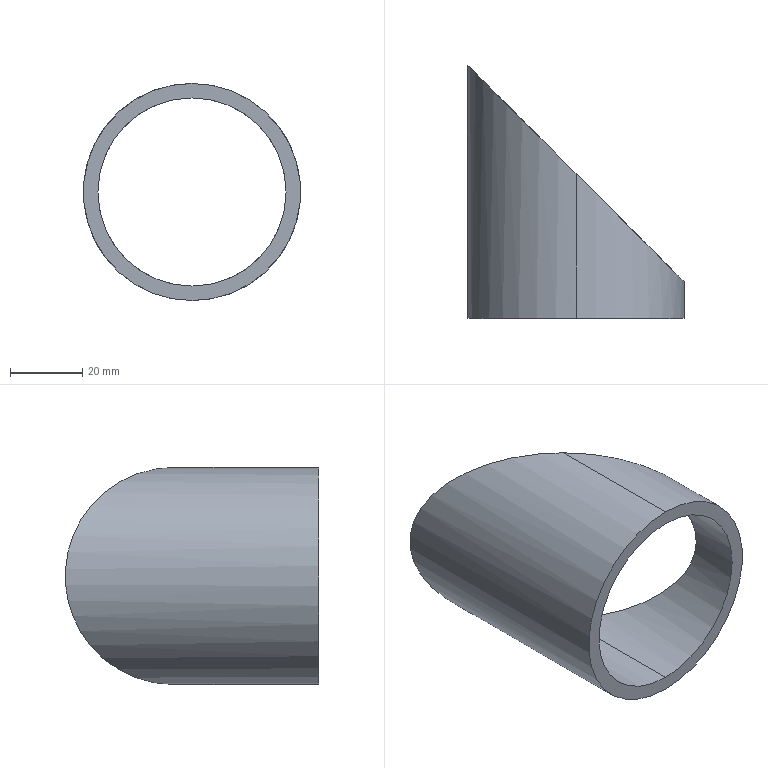Part | SolidWorks | features Extrusion 1, ICE 1 | 1 solid | 6 faces | box 60 x 70 x 60 mm | volume 28148 mm3 | cylinder 4 | plane 2 | commonest cylinder face diameters 52 x2 60 x2
STEP:
#1=CARTESIAN_POINT('',(0.,40.,-26.));
#2=VERTEX_POINT('',#1);
#3=CARTESIAN_POINT('',(0.,40.,26.));
#4=VERTEX_POINT('',#3);
#5=CARTESIAN_POINT('',(0.,40.,-26.));
#6=CARTESIAN_POINT('',(-52.,92.,-26.));
#7=CARTESIAN_POINT('',(-52.,92.,26.));
#8=CARTESIAN_POINT('',(0.,40.,26.));
#9=(BOUNDED_CURVE()B_SPLINE_CURVE(3,(#5,#6,#7,#8),.UNSPECIFIED.,.F.,.F.)B_SPLINE_CURVE_WITH_KNOTS((4,4),(1.571,4.712),.UNSPECIFIED.)CURVE()GEOMETRIC_REPRESENTATION_ITEM()RATIONAL_B_SPLINE_CURVE((1.,0.3333,0.3333,1.))REPRESENTATION_ITEM(''));
#10=EDGE_CURVE('',#2,#4,#9,.T.);
#11=ORIENTED_EDGE('',*,*,#10,.T.);
#12=CARTESIAN_POINT('',(0.,0.,26.));
#13=VERTEX_POINT('',#12);
#14=CARTESIAN_POINT('',(0.,70.,26.));
#15=DIRECTION('',(0.,-1.,0.));
#16=VECTOR('',#15,1000.);
#17=LINE('',#14,#16);
#18=EDGE_CURVE('',#4,#13,#17,.T.);
#19=ORIENTED_EDGE('',*,*,#18,.T.);
#20=CARTESIAN_POINT('',(0.,0.,-26.));
#21=VERTEX_POINT('',#20);
#22=CARTESIAN_POINT('',(0.,0.,0.));
#23=DIRECTION('',(0.,1.,0.));
#24=DIRECTION('',(0.,0.,1.));
#25=AXIS2_PLACEMENT_3D('',#22,#23,#24);
#26=CIRCLE('',#25,26.);
#27=EDGE_CURVE('',#21,#13,#26,.T.);
#28=ORIENTED_EDGE('',*,*,#27,.F.);
#29=CARTESIAN_POINT('',(0.,70.,-26.));
#30=DIRECTION('',(0.,-1.,0.));
#31=VECTOR('',#30,1000.);
#32=LINE('',#29,#31);
#33=EDGE_CURVE('',#2,#21,#32,.T.);
#34=ORIENTED_EDGE('',*,*,#33,.F.);
#35=EDGE_LOOP('',(#11,#19,#28,#34));
#36=FACE_OUTER_BOUND('',#35,.T.);
#37=CARTESIAN_POINT('',(0.,70.,0.));
#38=DIRECTION('',(0.,-1.,0.));
#39=DIRECTION('',(0.,0.,-1.));
#40=AXIS2_PLACEMENT_3D('',#37,#38,#39);
#41=CYLINDRICAL_SURFACE('',#40,26.);
#42=ADVANCED_FACE('',(#36),#41,.F.);
#43=CARTESIAN_POINT('',(0.,40.,30.));
#44=VERTEX_POINT('',#43);
#45=CARTESIAN_POINT('',(0.,40.,-30.));
#46=VERTEX_POINT('',#45);
#47=CARTESIAN_POINT('',(0.,40.,30.));
#48=CARTESIAN_POINT('',(60.,-20.,30.));
#49=CARTESIAN_POINT('',(60.,-20.,-30.));
#50=CARTESIAN_POINT('',(0.,40.,-30.));
#51=(BOUNDED_CURVE()B_SPLINE_CURVE(3,(#47,#48,#49,#50),.UNSPECIFIED.,.F.,.F.)B_SPLINE_CURVE_WITH_KNOTS((4,4),(4.712,7.854),.UNSPECIFIED.)CURVE()GEOMETRIC_REPRESENTATION_ITEM()RATIONAL_B_SPLINE_CURVE((1.,0.3333,0.3333,1.))REPRESENTATION_ITEM(''));
#52=EDGE_CURVE('',#44,#46,#51,.T.);
#53=ORIENTED_EDGE('',*,*,#52,.F.);
#54=CARTESIAN_POINT('',(0.,0.,30.));
#55=VERTEX_POINT('',#54);
#56=CARTESIAN_POINT('',(0.,70.,30.));
#57=DIRECTION('',(0.,-1.,0.));
#58=VECTOR('',#57,1000.);
#59=LINE('',#56,#58);
#60=EDGE_CURVE('',#44,#55,#59,.T.);
#61=ORIENTED_EDGE('',*,*,#60,.T.);
#62=CARTESIAN_POINT('',(0.,0.,-30.));
#63=VERTEX_POINT('',#62);
#64=CARTESIAN_POINT('',(0.,0.,0.));
#65=DIRECTION('',(0.,1.,0.));
#66=DIRECTION('',(0.,0.,1.));
#67=AXIS2_PLACEMENT_3D('',#64,#65,#66);
#68=CIRCLE('',#67,30.);
#69=EDGE_CURVE('',#55,#63,#68,.T.);
#70=ORIENTED_EDGE('',*,*,#69,.T.);
#71=CARTESIAN_POINT('',(0.,70.,-30.));
#72=DIRECTION('',(0.,-1.,0.));
#73=VECTOR('',#72,1000.);
#74=LINE('',#71,#73);
#75=EDGE_CURVE('',#46,#63,#74,.T.);
#76=ORIENTED_EDGE('',*,*,#75,.F.);
#77=EDGE_LOOP('',(#53,#61,#70,#76));
#78=FACE_OUTER_BOUND('',#77,.T.);
#79=CARTESIAN_POINT('',(0.,70.,0.));
#80=DIRECTION('',(0.,-1.,0.));
#81=DIRECTION('',(0.,0.,-1.));
#82=AXIS2_PLACEMENT_3D('',#79,#80,#81);
#83=CYLINDRICAL_SURFACE('',#82,30.);
#84=ADVANCED_FACE('',(#78),#83,.T.);
#85=ORIENTED_EDGE('',*,*,#60,.F.);
#86=CARTESIAN_POINT('',(0.,40.,-30.));
#87=CARTESIAN_POINT('',(-60.,100.,-30.));
#88=CARTESIAN_POINT('',(-60.,100.,30.));
#89=CARTESIAN_POINT('',(0.,40.,30.));
#90=(BOUNDED_CURVE()B_SPLINE_CURVE(3,(#86,#87,#88,#89),.UNSPECIFIED.,.F.,.F.)B_SPLINE_CURVE_WITH_KNOTS((4,4),(1.571,4.712),.UNSPECIFIED.)CURVE()GEOMETRIC_REPRESENTATION_ITEM()RATIONAL_B_SPLINE_CURVE((1.,0.3333,0.3333,1.))REPRESENTATION_ITEM(''));
#91=EDGE_CURVE('',#46,#44,#90,.T.);
#92=ORIENTED_EDGE('',*,*,#91,.F.);
#93=ORIENTED_EDGE('',*,*,#75,.T.);
#94=CARTESIAN_POINT('',(0.,0.,0.));
#95=DIRECTION('',(0.,1.,0.));
#96=DIRECTION('',(0.,0.,1.));
#97=AXIS2_PLACEMENT_3D('',#94,#95,#96);
#98=CIRCLE('',#97,30.);
#99=EDGE_CURVE('',#63,#55,#98,.T.);
#100=ORIENTED_EDGE('',*,*,#99,.T.);
#101=EDGE_LOOP('',(#85,#92,#93,#100));
#102=FACE_OUTER_BOUND('',#101,.T.);
#103=CARTESIAN_POINT('',(0.,70.,0.));
#104=DIRECTION('',(0.,-1.,0.));
#105=DIRECTION('',(0.,0.,-1.));
#106=AXIS2_PLACEMENT_3D('',#103,#104,#105);
#107=CYLINDRICAL_SURFACE('',#106,30.);
#108=ADVANCED_FACE('',(#102),#107,.T.);
#109=ORIENTED_EDGE('',*,*,#18,.F.);
#110=CARTESIAN_POINT('',(0.,40.,26.));
#111=CARTESIAN_POINT('',(52.,-12.,26.));
#112=CARTESIAN_POINT('',(52.,-12.,-26.));
#113=CARTESIAN_POINT('',(0.,40.,-26.));
#114=(BOUNDED_CURVE()B_SPLINE_CURVE(3,(#110,#111,#112,#113),.UNSPECIFIED.,.F.,.F.)B_SPLINE_CURVE_WITH_KNOTS((4,4),(4.712,7.854),.UNSPECIFIED.)CURVE()GEOMETRIC_REPRESENTATION_ITEM()RATIONAL_B_SPLINE_CURVE((1.,0.3333,0.3333,1.))REPRESENTATION_ITEM(''));
#115=EDGE_CURVE('',#4,#2,#114,.T.);
#116=ORIENTED_EDGE('',*,*,#115,.T.);
#117=ORIENTED_EDGE('',*,*,#33,.T.);
#118=CARTESIAN_POINT('',(0.,0.,0.));
#119=DIRECTION('',(0.,1.,0.));
#120=DIRECTION('',(0.,0.,1.));
#121=AXIS2_PLACEMENT_3D('',#118,#119,#120);
#122=CIRCLE('',#121,26.);
#123=EDGE_CURVE('',#13,#21,#122,.T.);
#124=ORIENTED_EDGE('',*,*,#123,.F.);
#125=EDGE_LOOP('',(#109,#116,#117,#124));
#126=FACE_OUTER_BOUND('',#125,.T.);
#127=CARTESIAN_POINT('',(0.,70.,0.));
#128=DIRECTION('',(0.,-1.,0.));
#129=DIRECTION('',(0.,0.,-1.));
#130=AXIS2_PLACEMENT_3D('',#127,#128,#129);
#131=CYLINDRICAL_SURFACE('',#130,26.);
#132=ADVANCED_FACE('',(#126),#131,.F.);
#133=ORIENTED_EDGE('',*,*,#99,.F.);
#134=ORIENTED_EDGE('',*,*,#69,.F.);
#135=EDGE_LOOP('',(#133,#134));
#136=FACE_OUTER_BOUND('',#135,.T.);
#137=ORIENTED_EDGE('',*,*,#27,.T.);
#138=ORIENTED_EDGE('',*,*,#123,.T.);
#139=EDGE_LOOP('',(#137,#138));
#140=FACE_BOUND('',#139,.T.);
#141=CARTESIAN_POINT('',(0.,0.,0.));
#142=DIRECTION('',(0.,1.,0.));
#143=DIRECTION('',(0.,0.,1.));
#144=AXIS2_PLACEMENT_3D('',#141,#142,#143);
#145=PLANE('',#144);
#146=ADVANCED_FACE('',(#136,#140),#145,.F.);
#147=ORIENTED_EDGE('',*,*,#10,.F.);
#148=ORIENTED_EDGE('',*,*,#115,.F.);
#149=EDGE_LOOP('',(#147,#148));
#150=FACE_BOUND('',#149,.T.);
#151=ORIENTED_EDGE('',*,*,#91,.T.);
#152=ORIENTED_EDGE('',*,*,#52,.T.);
#153=EDGE_LOOP('',(#151,#152));
#154=FACE_OUTER_BOUND('',#153,.T.);
#155=CARTESIAN_POINT('',(-30.,70.,175.));
#156=DIRECTION('',(0.7071,0.7071,0.));
#157=DIRECTION('',(-0.7071,0.7071,0.));
#158=AXIS2_PLACEMENT_3D('',#155,#156,#157);
#159=PLANE('',#158);
#160=ADVANCED_FACE('',(#150,#154),#159,.T.);
#161=CLOSED_SHELL('',(#42,#84,#108,#132,#146,#160));
#162=MANIFOLD_SOLID_BREP('',#161);
#163=CARTESIAN_POINT('',(0.,0.,0.));
#164=DIRECTION('',(0.,0.,1.));
#165=DIRECTION('',(1.,0.,0.));
#166=AXIS2_PLACEMENT_3D('',#163,#164,#165);
#167=(LENGTH_UNIT()NAMED_UNIT(*)SI_UNIT(.MILLI.,.METRE.));
#168=UNCERTAINTY_MEASURE_WITH_UNIT(LENGTH_MEASURE(0.00001),#167,'','');
#169=(NAMED_UNIT(*)PLANE_ANGLE_UNIT()SI_UNIT($,.RADIAN.));
#170=(NAMED_UNIT(*)SI_UNIT($,.STERADIAN.)SOLID_ANGLE_UNIT());
#171=(GEOMETRIC_REPRESENTATION_CONTEXT(3)GLOBAL_UNCERTAINTY_ASSIGNED_CONTEXT((#168))GLOBAL_UNIT_ASSIGNED_CONTEXT((#167,#169,#170))REPRESENTATION_CONTEXT('',''));
#172=ADVANCED_BREP_SHAPE_REPRESENTATION('',(#162,#166),#171);